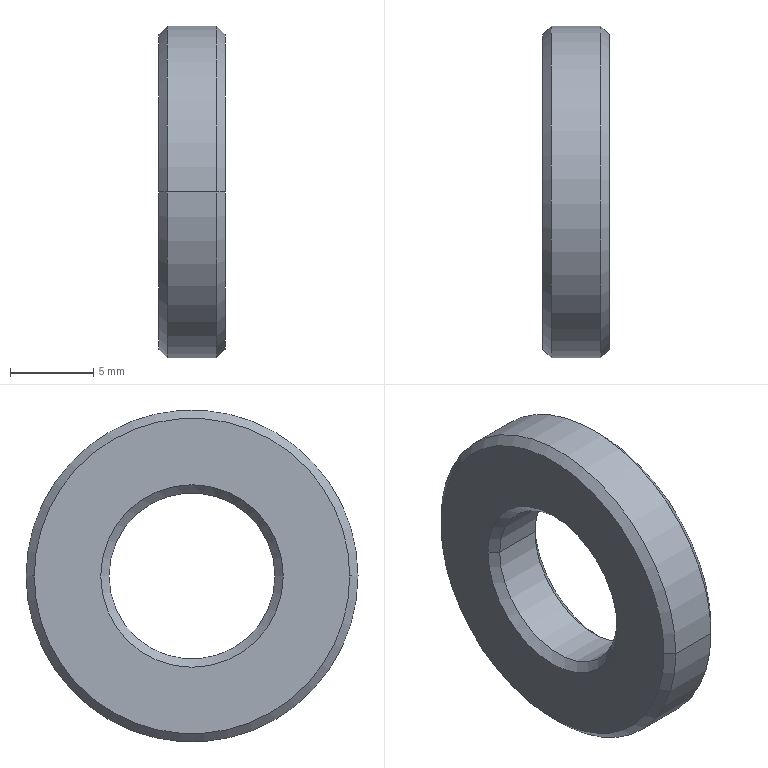Part | STEP file | WSSS20-10-4 | 1 solid | 14 faces | box 4 x 20 x 20 mm | volume 918.916 mm3 | cone 8 | cylinder 4 | plane 2 | commonest cylinder face diameters 10 x2 20 x2
STEP:
#1=CARTESIAN_POINT('',(0.,0.,0.));
#2=DIRECTION('',(0.,0.,1.));
#3=DIRECTION('',(1.,0.,0.));
#4=AXIS2_PLACEMENT_3D('',#1,#2,#3);
#5=CARTESIAN_POINT('',(3.5,-5.,0.));
#6=VERTEX_POINT('',#5);
#7=CARTESIAN_POINT('',(0.5,-5.,0.));
#8=VERTEX_POINT('',#7);
#9=CARTESIAN_POINT('',(-3.,-5.,0.));
#10=DIRECTION('',(-1.,0.,0.));
#11=VECTOR('',#10,1.);
#12=LINE('',#9,#11);
#13=CARTESIAN_POINT('',(-3.,0.,0.));
#14=DIRECTION('',(-1.,0.,0.));
#15=DIRECTION('',(0.,-1.,0.));
#16=AXIS2_PLACEMENT_3D('',#13,#14,#15);
#17=CYLINDRICAL_SURFACE('',#16,5.);
#18=CARTESIAN_POINT('',(6.283,0.));
#19=DIRECTION('',(0.,1.));
#20=VECTOR('',#19,1.);
#21=LINE('',#18,#20);
#22=(GEOMETRIC_REPRESENTATION_CONTEXT(2)PARAMETRIC_REPRESENTATION_CONTEXT()REPRESENTATION_CONTEXT('',''));
#23=DEFINITIONAL_REPRESENTATION('',(#21),#22);
#24=PCURVE('',#17,#23);
#25=CARTESIAN_POINT('',(-3.,0.,0.));
#26=DIRECTION('',(-1.,0.,0.));
#27=DIRECTION('',(0.,-1.,0.));
#28=AXIS2_PLACEMENT_3D('',#25,#26,#27);
#29=CYLINDRICAL_SURFACE('',#28,5.);
#30=CARTESIAN_POINT('',(0.,0.));
#31=DIRECTION('',(0.,1.));
#32=VECTOR('',#31,1.);
#33=LINE('',#30,#32);
#34=(GEOMETRIC_REPRESENTATION_CONTEXT(2)PARAMETRIC_REPRESENTATION_CONTEXT()REPRESENTATION_CONTEXT('',''));
#35=DEFINITIONAL_REPRESENTATION('',(#33),#34);
#36=PCURVE('',#29,#35);
#37=SURFACE_CURVE('',#12,(#24,#36),.PCURVE_S1.);
#38=EDGE_CURVE('',#6,#8,#37,.T.);
#39=ORIENTED_EDGE('',*,*,#38,.T.);
#40=CARTESIAN_POINT('',(0.5,5.,0.));
#41=VERTEX_POINT('',#40);
#42=CARTESIAN_POINT('',(0.5,0.,0.));
#43=DIRECTION('',(-1.,0.,0.));
#44=DIRECTION('',(0.,-1.,0.));
#45=AXIS2_PLACEMENT_3D('',#42,#43,#44);
#46=CIRCLE('',#45,5.);
#47=CARTESIAN_POINT('',(0.,-3.5));
#48=DIRECTION('',(1.,0.));
#49=VECTOR('',#48,1.);
#50=LINE('',#47,#49);
#51=(GEOMETRIC_REPRESENTATION_CONTEXT(2)PARAMETRIC_REPRESENTATION_CONTEXT()REPRESENTATION_CONTEXT('',''));
#52=DEFINITIONAL_REPRESENTATION('',(#50),#51);
#53=PCURVE('',#17,#52);
#54=CARTESIAN_POINT('',(0.5,0.,0.));
#55=DIRECTION('',(-1.,0.,0.));
#56=DIRECTION('',(0.,-1.,0.));
#57=AXIS2_PLACEMENT_3D('',#54,#55,#56);
#58=CONICAL_SURFACE('',#57,5.,0.7854);
#59=CARTESIAN_POINT('',(0.,0.));
#60=DIRECTION('',(1.,0.));
#61=VECTOR('',#60,1.);
#62=LINE('',#59,#61);
#63=(GEOMETRIC_REPRESENTATION_CONTEXT(2)PARAMETRIC_REPRESENTATION_CONTEXT()REPRESENTATION_CONTEXT('',''));
#64=DEFINITIONAL_REPRESENTATION('',(#62),#63);
#65=PCURVE('',#58,#64);
#66=SURFACE_CURVE('',#46,(#53,#65),.PCURVE_S1.);
#67=EDGE_CURVE('',#41,#8,#66,.T.);
#68=ORIENTED_EDGE('',*,*,#67,.F.);
#69=CARTESIAN_POINT('',(3.5,5.,0.));
#70=VERTEX_POINT('',#69);
#71=CARTESIAN_POINT('',(-3.,5.,0.));
#72=DIRECTION('',(-1.,0.,0.));
#73=VECTOR('',#72,1.);
#74=LINE('',#71,#73);
#75=CARTESIAN_POINT('',(3.142,0.));
#76=DIRECTION('',(0.,1.));
#77=VECTOR('',#76,1.);
#78=LINE('',#75,#77);
#79=(GEOMETRIC_REPRESENTATION_CONTEXT(2)PARAMETRIC_REPRESENTATION_CONTEXT()REPRESENTATION_CONTEXT('',''));
#80=DEFINITIONAL_REPRESENTATION('',(#78),#79);
#81=PCURVE('',#17,#80);
#82=CARTESIAN_POINT('',(3.142,0.));
#83=DIRECTION('',(0.,1.));
#84=VECTOR('',#83,1.);
#85=LINE('',#82,#84);
#86=(GEOMETRIC_REPRESENTATION_CONTEXT(2)PARAMETRIC_REPRESENTATION_CONTEXT()REPRESENTATION_CONTEXT('',''));
#87=DEFINITIONAL_REPRESENTATION('',(#85),#86);
#88=PCURVE('',#29,#87);
#89=SURFACE_CURVE('',#74,(#81,#88),.PCURVE_S1.);
#90=EDGE_CURVE('',#70,#41,#89,.T.);
#91=ORIENTED_EDGE('',*,*,#90,.F.);
#92=CARTESIAN_POINT('',(3.5,0.,0.));
#93=DIRECTION('',(-1.,0.,0.));
#94=DIRECTION('',(0.,-1.,0.));
#95=AXIS2_PLACEMENT_3D('',#92,#93,#94);
#96=CIRCLE('',#95,5.);
#97=CARTESIAN_POINT('',(0.,-6.5));
#98=DIRECTION('',(1.,0.));
#99=VECTOR('',#98,1.);
#100=LINE('',#97,#99);
#101=(GEOMETRIC_REPRESENTATION_CONTEXT(2)PARAMETRIC_REPRESENTATION_CONTEXT()REPRESENTATION_CONTEXT('',''));
#102=DEFINITIONAL_REPRESENTATION('',(#100),#101);
#103=PCURVE('',#17,#102);
#104=CARTESIAN_POINT('',(4.,0.,0.));
#105=DIRECTION('',(1.,0.,0.));
#106=DIRECTION('',(0.,1.,0.));
#107=AXIS2_PLACEMENT_3D('',#104,#105,#106);
#108=CONICAL_SURFACE('',#107,5.5,0.7854);
#109=CARTESIAN_POINT('',(9.425,-0.5));
#110=DIRECTION('',(-1.,0.));
#111=VECTOR('',#110,1.);
#112=LINE('',#109,#111);
#113=(GEOMETRIC_REPRESENTATION_CONTEXT(2)PARAMETRIC_REPRESENTATION_CONTEXT()REPRESENTATION_CONTEXT('',''));
#114=DEFINITIONAL_REPRESENTATION('',(#112),#113);
#115=PCURVE('',#108,#114);
#116=SURFACE_CURVE('',#96,(#103,#115),.PCURVE_S1.);
#117=EDGE_CURVE('',#70,#6,#116,.T.);
#118=ORIENTED_EDGE('',*,*,#117,.T.);
#119=EDGE_LOOP('',(#39,#68,#91,#118));
#120=FACE_BOUND('',#119,.F.);
#121=ADVANCED_FACE('',(#120),#17,.F.);
#122=CARTESIAN_POINT('',(4.,5.5,0.));
#123=VERTEX_POINT('',#122);
#124=CARTESIAN_POINT('',(4.,5.5,0.));
#125=DIRECTION('',(0.7071,0.7071,0.));
#126=VECTOR('',#125,1.);
#127=LINE('',#124,#126);
#128=CARTESIAN_POINT('',(6.283,0.));
#129=DIRECTION('',(0.,1.));
#130=VECTOR('',#129,1.);
#131=LINE('',#128,#130);
#132=(GEOMETRIC_REPRESENTATION_CONTEXT(2)PARAMETRIC_REPRESENTATION_CONTEXT()REPRESENTATION_CONTEXT('',''));
#133=DEFINITIONAL_REPRESENTATION('',(#131),#132);
#134=PCURVE('',#108,#133);
#135=CARTESIAN_POINT('',(4.,0.,0.));
#136=DIRECTION('',(1.,0.,0.));
#137=DIRECTION('',(0.,1.,0.));
#138=AXIS2_PLACEMENT_3D('',#135,#136,#137);
#139=CONICAL_SURFACE('',#138,5.5,0.7854);
#140=CARTESIAN_POINT('',(0.,0.));
#141=DIRECTION('',(0.,1.));
#142=VECTOR('',#141,1.);
#143=LINE('',#140,#142);
#144=(GEOMETRIC_REPRESENTATION_CONTEXT(2)PARAMETRIC_REPRESENTATION_CONTEXT()REPRESENTATION_CONTEXT('',''));
#145=DEFINITIONAL_REPRESENTATION('',(#143),#144);
#146=PCURVE('',#139,#145);
#147=SURFACE_CURVE('',#127,(#134,#146),.PCURVE_S1.);
#148=EDGE_CURVE('',#70,#123,#147,.T.);
#149=ORIENTED_EDGE('',*,*,#148,.T.);
#150=CARTESIAN_POINT('',(4.,-5.5,0.));
#151=VERTEX_POINT('',#150);
#152=CARTESIAN_POINT('',(4.,0.,0.));
#153=DIRECTION('',(-1.,0.,0.));
#154=DIRECTION('',(0.,-1.,0.));
#155=AXIS2_PLACEMENT_3D('',#152,#153,#154);
#156=CIRCLE('',#155,5.5);
#157=CARTESIAN_POINT('',(9.425,0.));
#158=DIRECTION('',(-1.,0.));
#159=VECTOR('',#158,1.);
#160=LINE('',#157,#159);
#161=(GEOMETRIC_REPRESENTATION_CONTEXT(2)PARAMETRIC_REPRESENTATION_CONTEXT()REPRESENTATION_CONTEXT('',''));
#162=DEFINITIONAL_REPRESENTATION('',(#160),#161);
#163=PCURVE('',#108,#162);
#164=CARTESIAN_POINT('',(4.,-9.5,0.));
#165=DIRECTION('',(1.,0.,0.));
#166=DIRECTION('',(0.,1.,0.));
#167=AXIS2_PLACEMENT_3D('',#164,#165,#166);
#168=PLANE('',#167);
#169=CARTESIAN_POINT('',(4.,0.));
#170=CARTESIAN_POINT('',(4.,9.526));
#171=CARTESIAN_POINT('',(12.25,4.763));
#172=CARTESIAN_POINT('',(20.5,0.));
#173=CARTESIAN_POINT('',(12.25,-4.763));
#174=CARTESIAN_POINT('',(4.,-9.526));
#175=CARTESIAN_POINT('',(4.,0.));
#176=(BOUNDED_CURVE()B_SPLINE_CURVE(2,(#169,#170,#171,#172,#173,#174,#175),.UNSPECIFIED.,.T.,.F.)B_SPLINE_CURVE_WITH_KNOTS((1,2,2,2,2,1),(-2.094,0.,2.094,4.189,6.283,8.378),.UNSPECIFIED.)CURVE()GEOMETRIC_REPRESENTATION_ITEM()RATIONAL_B_SPLINE_CURVE((1.,0.5,1.,0.5,1.,0.5,1.))REPRESENTATION_ITEM(''));
#177=(GEOMETRIC_REPRESENTATION_CONTEXT(2)PARAMETRIC_REPRESENTATION_CONTEXT()REPRESENTATION_CONTEXT('',''));
#178=DEFINITIONAL_REPRESENTATION('',(#176),#177);
#179=PCURVE('',#168,#178);
#180=SURFACE_CURVE('',#156,(#163,#179),.PCURVE_S1.);
#181=EDGE_CURVE('',#123,#151,#180,.T.);
#182=ORIENTED_EDGE('',*,*,#181,.T.);
#183=CARTESIAN_POINT('',(4.,-5.5,0.));
#184=DIRECTION('',(0.7071,-0.7071,0.));
#185=VECTOR('',#184,1.);
#186=LINE('',#183,#185);
#187=CARTESIAN_POINT('',(3.142,0.));
#188=DIRECTION('',(0.,1.));
#189=VECTOR('',#188,1.);
#190=LINE('',#187,#189);
#191=(GEOMETRIC_REPRESENTATION_CONTEXT(2)PARAMETRIC_REPRESENTATION_CONTEXT()REPRESENTATION_CONTEXT('',''));
#192=DEFINITIONAL_REPRESENTATION('',(#190),#191);
#193=PCURVE('',#108,#192);
#194=CARTESIAN_POINT('',(3.142,0.));
#195=DIRECTION('',(0.,1.));
#196=VECTOR('',#195,1.);
#197=LINE('',#194,#196);
#198=(GEOMETRIC_REPRESENTATION_CONTEXT(2)PARAMETRIC_REPRESENTATION_CONTEXT()REPRESENTATION_CONTEXT('',''));
#199=DEFINITIONAL_REPRESENTATION('',(#197),#198);
#200=PCURVE('',#139,#199);
#201=SURFACE_CURVE('',#186,(#193,#200),.PCURVE_S1.);
#202=EDGE_CURVE('',#6,#151,#201,.T.);
#203=ORIENTED_EDGE('',*,*,#202,.F.);
#204=ORIENTED_EDGE('',*,*,#117,.F.);
#205=EDGE_LOOP('',(#149,#182,#203,#204));
#206=FACE_BOUND('',#205,.F.);
#207=ADVANCED_FACE('',(#206),#108,.F.);
#208=CARTESIAN_POINT('',(4.,-9.5,0.));
#209=VERTEX_POINT('',#208);
#210=CARTESIAN_POINT('',(4.,9.5,0.));
#211=VERTEX_POINT('',#210);
#212=CARTESIAN_POINT('',(4.,0.,0.));
#213=DIRECTION('',(-1.,0.,0.));
#214=DIRECTION('',(0.,-1.,0.));
#215=AXIS2_PLACEMENT_3D('',#212,#213,#214);
#216=CIRCLE('',#215,9.5);
#217=CARTESIAN_POINT('',(3.5,0.,0.));
#218=DIRECTION('',(-1.,0.,0.));
#219=DIRECTION('',(0.,-1.,0.));
#220=AXIS2_PLACEMENT_3D('',#217,#218,#219);
#221=CONICAL_SURFACE('',#220,10.,0.7854);
#222=CARTESIAN_POINT('',(0.,-0.5));
#223=DIRECTION('',(1.,0.));
#224=VECTOR('',#223,1.);
#225=LINE('',#222,#224);
#226=(GEOMETRIC_REPRESENTATION_CONTEXT(2)PARAMETRIC_REPRESENTATION_CONTEXT()REPRESENTATION_CONTEXT('',''));
#227=DEFINITIONAL_REPRESENTATION('',(#225),#226);
#228=PCURVE('',#221,#227);
#229=CARTESIAN_POINT('',(0.,0.));
#230=CARTESIAN_POINT('',(0.,16.454));
#231=CARTESIAN_POINT('',(14.25,8.227));
#232=CARTESIAN_POINT('',(28.5,0.));
#233=CARTESIAN_POINT('',(14.25,-8.227));
#234=CARTESIAN_POINT('',(0.,-16.454));
#235=CARTESIAN_POINT('',(0.,0.));
#236=(BOUNDED_CURVE()B_SPLINE_CURVE(2,(#229,#230,#231,#232,#233,#234,#235),.UNSPECIFIED.,.T.,.F.)B_SPLINE_CURVE_WITH_KNOTS((1,2,2,2,2,1),(-2.094,0.,2.094,4.189,6.283,8.378),.UNSPECIFIED.)CURVE()GEOMETRIC_REPRESENTATION_ITEM()RATIONAL_B_SPLINE_CURVE((1.,0.5,1.,0.5,1.,0.5,1.))REPRESENTATION_ITEM(''));
#237=(GEOMETRIC_REPRESENTATION_CONTEXT(2)PARAMETRIC_REPRESENTATION_CONTEXT()REPRESENTATION_CONTEXT('',''));
#238=DEFINITIONAL_REPRESENTATION('',(#236),#237);
#239=PCURVE('',#168,#238);
#240=SURFACE_CURVE('',#216,(#228,#239),.PCURVE_S1.);
#241=EDGE_CURVE('',#209,#211,#240,.T.);
#242=ORIENTED_EDGE('',*,*,#241,.T.);
#243=CARTESIAN_POINT('',(3.5,10.,0.));
#244=VERTEX_POINT('',#243);
#245=CARTESIAN_POINT('',(3.5,10.,0.));
#246=DIRECTION('',(-0.7071,0.7071,0.));
#247=VECTOR('',#246,1.);
#248=LINE('',#245,#247);
#249=CARTESIAN_POINT('',(3.142,0.));
#250=DIRECTION('',(0.,1.));
#251=VECTOR('',#250,1.);
#252=LINE('',#249,#251);
#253=(GEOMETRIC_REPRESENTATION_CONTEXT(2)PARAMETRIC_REPRESENTATION_CONTEXT()REPRESENTATION_CONTEXT('',''));
#254=DEFINITIONAL_REPRESENTATION('',(#252),#253);
#255=PCURVE('',#221,#254);
#256=CARTESIAN_POINT('',(3.5,0.,0.));
#257=DIRECTION('',(-1.,0.,0.));
#258=DIRECTION('',(0.,-1.,0.));
#259=AXIS2_PLACEMENT_3D('',#256,#257,#258);
#260=CONICAL_SURFACE('',#259,10.,0.7854);
#261=CARTESIAN_POINT('',(3.142,0.));
#262=DIRECTION('',(0.,1.));
#263=VECTOR('',#262,1.);
#264=LINE('',#261,#263);
#265=(GEOMETRIC_REPRESENTATION_CONTEXT(2)PARAMETRIC_REPRESENTATION_CONTEXT()REPRESENTATION_CONTEXT('',''));
#266=DEFINITIONAL_REPRESENTATION('',(#264),#265);
#267=PCURVE('',#260,#266);
#268=SURFACE_CURVE('',#248,(#255,#267),.PCURVE_S1.);
#269=EDGE_CURVE('',#211,#244,#268,.T.);
#270=ORIENTED_EDGE('',*,*,#269,.T.);
#271=CARTESIAN_POINT('',(3.5,-10.,0.));
#272=VERTEX_POINT('',#271);
#273=CARTESIAN_POINT('',(3.5,0.,0.));
#274=DIRECTION('',(-1.,0.,0.));
#275=DIRECTION('',(0.,-1.,0.));
#276=AXIS2_PLACEMENT_3D('',#273,#274,#275);
#277=CIRCLE('',#276,10.);
#278=CARTESIAN_POINT('',(0.,0.));
#279=DIRECTION('',(1.,0.));
#280=VECTOR('',#279,1.);
#281=LINE('',#278,#280);
#282=(GEOMETRIC_REPRESENTATION_CONTEXT(2)PARAMETRIC_REPRESENTATION_CONTEXT()REPRESENTATION_CONTEXT('',''));
#283=DEFINITIONAL_REPRESENTATION('',(#281),#282);
#284=PCURVE('',#221,#283);
#285=CARTESIAN_POINT('',(-3.,0.,0.));
#286=DIRECTION('',(-1.,0.,0.));
#287=DIRECTION('',(0.,-1.,0.));
#288=AXIS2_PLACEMENT_3D('',#285,#286,#287);
#289=CYLINDRICAL_SURFACE('',#288,10.);
#290=CARTESIAN_POINT('',(0.,-6.5));
#291=DIRECTION('',(1.,0.));
#292=VECTOR('',#291,1.);
#293=LINE('',#290,#292);
#294=(GEOMETRIC_REPRESENTATION_CONTEXT(2)PARAMETRIC_REPRESENTATION_CONTEXT()REPRESENTATION_CONTEXT('',''));
#295=DEFINITIONAL_REPRESENTATION('',(#293),#294);
#296=PCURVE('',#289,#295);
#297=SURFACE_CURVE('',#277,(#284,#296),.PCURVE_S1.);
#298=EDGE_CURVE('',#272,#244,#297,.T.);
#299=ORIENTED_EDGE('',*,*,#298,.F.);
#300=CARTESIAN_POINT('',(3.5,-10.,0.));
#301=DIRECTION('',(-0.7071,-0.7071,0.));
#302=VECTOR('',#301,1.);
#303=LINE('',#300,#302);
#304=CARTESIAN_POINT('',(0.,0.));
#305=DIRECTION('',(0.,1.));
#306=VECTOR('',#305,1.);
#307=LINE('',#304,#306);
#308=(GEOMETRIC_REPRESENTATION_CONTEXT(2)PARAMETRIC_REPRESENTATION_CONTEXT()REPRESENTATION_CONTEXT('',''));
#309=DEFINITIONAL_REPRESENTATION('',(#307),#308);
#310=PCURVE('',#221,#309);
#311=CARTESIAN_POINT('',(6.283,0.));
#312=DIRECTION('',(0.,1.));
#313=VECTOR('',#312,1.);
#314=LINE('',#311,#313);
#315=(GEOMETRIC_REPRESENTATION_CONTEXT(2)PARAMETRIC_REPRESENTATION_CONTEXT()REPRESENTATION_CONTEXT('',''));
#316=DEFINITIONAL_REPRESENTATION('',(#314),#315);
#317=PCURVE('',#260,#316);
#318=SURFACE_CURVE('',#303,(#310,#317),.PCURVE_S1.);
#319=EDGE_CURVE('',#209,#272,#318,.T.);
#320=ORIENTED_EDGE('',*,*,#319,.F.);
#321=EDGE_LOOP('',(#242,#270,#299,#320));
#322=FACE_BOUND('',#321,.T.);
#323=ADVANCED_FACE('',(#322),#221,.T.);
#324=ORIENTED_EDGE('',*,*,#298,.T.);
#325=CARTESIAN_POINT('',(0.5,10.,0.));
#326=VERTEX_POINT('',#325);
#327=CARTESIAN_POINT('',(-3.,10.,0.));
#328=DIRECTION('',(-1.,0.,0.));
#329=VECTOR('',#328,1.);
#330=LINE('',#327,#329);
#331=CARTESIAN_POINT('',(3.142,0.));
#332=DIRECTION('',(0.,1.));
#333=VECTOR('',#332,1.);
#334=LINE('',#331,#333);
#335=(GEOMETRIC_REPRESENTATION_CONTEXT(2)PARAMETRIC_REPRESENTATION_CONTEXT()REPRESENTATION_CONTEXT('',''));
#336=DEFINITIONAL_REPRESENTATION('',(#334),#335);
#337=PCURVE('',#289,#336);
#338=CARTESIAN_POINT('',(-3.,0.,0.));
#339=DIRECTION('',(-1.,0.,0.));
#340=DIRECTION('',(0.,-1.,0.));
#341=AXIS2_PLACEMENT_3D('',#338,#339,#340);
#342=CYLINDRICAL_SURFACE('',#341,10.);
#343=CARTESIAN_POINT('',(3.142,0.));
#344=DIRECTION('',(0.,1.));
#345=VECTOR('',#344,1.);
#346=LINE('',#343,#345);
#347=(GEOMETRIC_REPRESENTATION_CONTEXT(2)PARAMETRIC_REPRESENTATION_CONTEXT()REPRESENTATION_CONTEXT('',''));
#348=DEFINITIONAL_REPRESENTATION('',(#346),#347);
#349=PCURVE('',#342,#348);
#350=SURFACE_CURVE('',#330,(#337,#349),.PCURVE_S1.);
#351=EDGE_CURVE('',#244,#326,#350,.T.);
#352=ORIENTED_EDGE('',*,*,#351,.T.);
#353=CARTESIAN_POINT('',(0.5,-10.,0.));
#354=VERTEX_POINT('',#353);
#355=CARTESIAN_POINT('',(0.5,0.,0.));
#356=DIRECTION('',(-1.,0.,0.));
#357=DIRECTION('',(0.,-1.,0.));
#358=AXIS2_PLACEMENT_3D('',#355,#356,#357);
#359=CIRCLE('',#358,10.);
#360=CARTESIAN_POINT('',(0.,-3.5));
#361=DIRECTION('',(1.,0.));
#362=VECTOR('',#361,1.);
#363=LINE('',#360,#362);
#364=(GEOMETRIC_REPRESENTATION_CONTEXT(2)PARAMETRIC_REPRESENTATION_CONTEXT()REPRESENTATION_CONTEXT('',''));
#365=DEFINITIONAL_REPRESENTATION('',(#363),#364);
#366=PCURVE('',#289,#365);
#367=CARTESIAN_POINT('',(0.,0.,0.));
#368=DIRECTION('',(1.,0.,0.));
#369=DIRECTION('',(0.,1.,0.));
#370=AXIS2_PLACEMENT_3D('',#367,#368,#369);
#371=CONICAL_SURFACE('',#370,9.5,0.7854);
#372=CARTESIAN_POINT('',(3.142,0.5));
#373=DIRECTION('',(-1.,0.));
#374=VECTOR('',#373,1.);
#375=LINE('',#372,#374);
#376=(GEOMETRIC_REPRESENTATION_CONTEXT(2)PARAMETRIC_REPRESENTATION_CONTEXT()REPRESENTATION_CONTEXT('',''));
#377=DEFINITIONAL_REPRESENTATION('',(#375),#376);
#378=PCURVE('',#371,#377);
#379=SURFACE_CURVE('',#359,(#366,#378),.PCURVE_S1.);
#380=EDGE_CURVE('',#354,#326,#379,.T.);
#381=ORIENTED_EDGE('',*,*,#380,.F.);
#382=CARTESIAN_POINT('',(-3.,-10.,0.));
#383=DIRECTION('',(-1.,0.,0.));
#384=VECTOR('',#383,1.);
#385=LINE('',#382,#384);
#386=CARTESIAN_POINT('',(0.,0.));
#387=DIRECTION('',(0.,1.));
#388=VECTOR('',#387,1.);
#389=LINE('',#386,#388);
#390=(GEOMETRIC_REPRESENTATION_CONTEXT(2)PARAMETRIC_REPRESENTATION_CONTEXT()REPRESENTATION_CONTEXT('',''));
#391=DEFINITIONAL_REPRESENTATION('',(#389),#390);
#392=PCURVE('',#289,#391);
#393=CARTESIAN_POINT('',(6.283,0.));
#394=DIRECTION('',(0.,1.));
#395=VECTOR('',#394,1.);
#396=LINE('',#393,#395);
#397=(GEOMETRIC_REPRESENTATION_CONTEXT(2)PARAMETRIC_REPRESENTATION_CONTEXT()REPRESENTATION_CONTEXT('',''));
#398=DEFINITIONAL_REPRESENTATION('',(#396),#397);
#399=PCURVE('',#342,#398);
#400=SURFACE_CURVE('',#385,(#392,#399),.PCURVE_S1.);
#401=EDGE_CURVE('',#272,#354,#400,.T.);
#402=ORIENTED_EDGE('',*,*,#401,.F.);
#403=EDGE_LOOP('',(#324,#352,#381,#402));
#404=FACE_BOUND('',#403,.T.);
#405=ADVANCED_FACE('',(#404),#289,.T.);
#406=CARTESIAN_POINT('',(0.,-9.5,0.));
#407=VERTEX_POINT('',#406);
#408=CARTESIAN_POINT('',(0.,9.5,0.));
#409=VERTEX_POINT('',#408);
#410=CARTESIAN_POINT('',(0.,0.,0.));
#411=DIRECTION('',(-1.,0.,0.));
#412=DIRECTION('',(0.,-1.,0.));
#413=AXIS2_PLACEMENT_3D('',#410,#411,#412);
#414=CIRCLE('',#413,9.5);
#415=CARTESIAN_POINT('',(3.142,0.));
#416=DIRECTION('',(-1.,0.));
#417=VECTOR('',#416,1.);
#418=LINE('',#415,#417);
#419=(GEOMETRIC_REPRESENTATION_CONTEXT(2)PARAMETRIC_REPRESENTATION_CONTEXT()REPRESENTATION_CONTEXT('',''));
#420=DEFINITIONAL_REPRESENTATION('',(#418),#419);
#421=PCURVE('',#371,#420);
#422=CARTESIAN_POINT('',(0.,-5.5,0.));
#423=DIRECTION('',(-1.,0.,0.));
#424=DIRECTION('',(0.,-1.,0.));
#425=AXIS2_PLACEMENT_3D('',#422,#423,#424);
#426=PLANE('',#425);
#427=CARTESIAN_POINT('',(-5.5,0.));
#428=DIRECTION('',(1.,0.));
#429=AXIS2_PLACEMENT_2D('',#427,#428);
#430=CIRCLE('',#429,9.5);
#431=(GEOMETRIC_REPRESENTATION_CONTEXT(2)PARAMETRIC_REPRESENTATION_CONTEXT()REPRESENTATION_CONTEXT('',''));
#432=DEFINITIONAL_REPRESENTATION('',(#430),#431);
#433=PCURVE('',#426,#432);
#434=SURFACE_CURVE('',#414,(#421,#433),.PCURVE_S1.);
#435=EDGE_CURVE('',#407,#409,#434,.T.);
#436=ORIENTED_EDGE('',*,*,#435,.F.);
#437=CARTESIAN_POINT('',(0.,-9.5,0.));
#438=DIRECTION('',(0.7071,-0.7071,0.));
#439=VECTOR('',#438,1.);
#440=LINE('',#437,#439);
#441=CARTESIAN_POINT('',(3.142,0.));
#442=DIRECTION('',(0.,1.));
#443=VECTOR('',#442,1.);
#444=LINE('',#441,#443);
#445=(GEOMETRIC_REPRESENTATION_CONTEXT(2)PARAMETRIC_REPRESENTATION_CONTEXT()REPRESENTATION_CONTEXT('',''));
#446=DEFINITIONAL_REPRESENTATION('',(#444),#445);
#447=PCURVE('',#371,#446);
#448=CARTESIAN_POINT('',(0.,0.,0.));
#449=DIRECTION('',(1.,0.,0.));
#450=DIRECTION('',(0.,1.,0.));
#451=AXIS2_PLACEMENT_3D('',#448,#449,#450);
#452=CONICAL_SURFACE('',#451,9.5,0.7854);
#453=CARTESIAN_POINT('',(3.142,0.));
#454=DIRECTION('',(0.,1.));
#455=VECTOR('',#454,1.);
#456=LINE('',#453,#455);
#457=(GEOMETRIC_REPRESENTATION_CONTEXT(2)PARAMETRIC_REPRESENTATION_CONTEXT()REPRESENTATION_CONTEXT('',''));
#458=DEFINITIONAL_REPRESENTATION('',(#456),#457);
#459=PCURVE('',#452,#458);
#460=SURFACE_CURVE('',#440,(#447,#459),.PCURVE_S1.);
#461=EDGE_CURVE('',#407,#354,#460,.T.);
#462=ORIENTED_EDGE('',*,*,#461,.T.);
#463=ORIENTED_EDGE('',*,*,#380,.T.);
#464=CARTESIAN_POINT('',(0.,9.5,0.));
#465=DIRECTION('',(0.7071,0.7071,0.));
#466=VECTOR('',#465,1.);
#467=LINE('',#464,#466);
#468=CARTESIAN_POINT('',(0.,0.));
#469=DIRECTION('',(0.,1.));
#470=VECTOR('',#469,1.);
#471=LINE('',#468,#470);
#472=(GEOMETRIC_REPRESENTATION_CONTEXT(2)PARAMETRIC_REPRESENTATION_CONTEXT()REPRESENTATION_CONTEXT('',''));
#473=DEFINITIONAL_REPRESENTATION('',(#471),#472);
#474=PCURVE('',#371,#473);
#475=CARTESIAN_POINT('',(6.283,0.));
#476=DIRECTION('',(0.,1.));
#477=VECTOR('',#476,1.);
#478=LINE('',#475,#477);
#479=(GEOMETRIC_REPRESENTATION_CONTEXT(2)PARAMETRIC_REPRESENTATION_CONTEXT()REPRESENTATION_CONTEXT('',''));
#480=DEFINITIONAL_REPRESENTATION('',(#478),#479);
#481=PCURVE('',#452,#480);
#482=SURFACE_CURVE('',#467,(#474,#481),.PCURVE_S1.);
#483=EDGE_CURVE('',#409,#326,#482,.T.);
#484=ORIENTED_EDGE('',*,*,#483,.F.);
#485=EDGE_LOOP('',(#436,#462,#463,#484));
#486=FACE_BOUND('',#485,.T.);
#487=ADVANCED_FACE('',(#486),#371,.T.);
#488=CARTESIAN_POINT('',(0.,-5.5,0.));
#489=VERTEX_POINT('',#488);
#490=CARTESIAN_POINT('',(0.5,-5.,0.));
#491=DIRECTION('',(-0.7071,-0.7071,0.));
#492=VECTOR('',#491,1.);
#493=LINE('',#490,#492);
#494=CARTESIAN_POINT('',(6.283,0.));
#495=DIRECTION('',(0.,1.));
#496=VECTOR('',#495,1.);
#497=LINE('',#494,#496);
#498=(GEOMETRIC_REPRESENTATION_CONTEXT(2)PARAMETRIC_REPRESENTATION_CONTEXT()REPRESENTATION_CONTEXT('',''));
#499=DEFINITIONAL_REPRESENTATION('',(#497),#498);
#500=PCURVE('',#58,#499);
#501=CARTESIAN_POINT('',(0.5,0.,0.));
#502=DIRECTION('',(-1.,0.,0.));
#503=DIRECTION('',(0.,-1.,0.));
#504=AXIS2_PLACEMENT_3D('',#501,#502,#503);
#505=CONICAL_SURFACE('',#504,5.,0.7854);
#506=CARTESIAN_POINT('',(0.,0.));
#507=DIRECTION('',(0.,1.));
#508=VECTOR('',#507,1.);
#509=LINE('',#506,#508);
#510=(GEOMETRIC_REPRESENTATION_CONTEXT(2)PARAMETRIC_REPRESENTATION_CONTEXT()REPRESENTATION_CONTEXT('',''));
#511=DEFINITIONAL_REPRESENTATION('',(#509),#510);
#512=PCURVE('',#505,#511);
#513=SURFACE_CURVE('',#493,(#500,#512),.PCURVE_S1.);
#514=EDGE_CURVE('',#8,#489,#513,.T.);
#515=ORIENTED_EDGE('',*,*,#514,.T.);
#516=CARTESIAN_POINT('',(0.,5.5,0.));
#517=VERTEX_POINT('',#516);
#518=CARTESIAN_POINT('',(0.,0.,0.));
#519=DIRECTION('',(-1.,0.,0.));
#520=DIRECTION('',(0.,-1.,0.));
#521=AXIS2_PLACEMENT_3D('',#518,#519,#520);
#522=CIRCLE('',#521,5.5);
#523=CARTESIAN_POINT('',(0.,0.5));
#524=DIRECTION('',(1.,0.));
#525=VECTOR('',#524,1.);
#526=LINE('',#523,#525);
#527=(GEOMETRIC_REPRESENTATION_CONTEXT(2)PARAMETRIC_REPRESENTATION_CONTEXT()REPRESENTATION_CONTEXT('',''));
#528=DEFINITIONAL_REPRESENTATION('',(#526),#527);
#529=PCURVE('',#58,#528);
#530=CARTESIAN_POINT('',(-5.5,0.));
#531=DIRECTION('',(1.,0.));
#532=AXIS2_PLACEMENT_2D('',#530,#531);
#533=CIRCLE('',#532,5.5);
#534=(GEOMETRIC_REPRESENTATION_CONTEXT(2)PARAMETRIC_REPRESENTATION_CONTEXT()REPRESENTATION_CONTEXT('',''));
#535=DEFINITIONAL_REPRESENTATION('',(#533),#534);
#536=PCURVE('',#426,#535);
#537=SURFACE_CURVE('',#522,(#529,#536),.PCURVE_S1.);
#538=EDGE_CURVE('',#517,#489,#537,.T.);
#539=ORIENTED_EDGE('',*,*,#538,.F.);
#540=CARTESIAN_POINT('',(0.5,5.,0.));
#541=DIRECTION('',(-0.7071,0.7071,0.));
#542=VECTOR('',#541,1.);
#543=LINE('',#540,#542);
#544=CARTESIAN_POINT('',(3.142,0.));
#545=DIRECTION('',(0.,1.));
#546=VECTOR('',#545,1.);
#547=LINE('',#544,#546);
#548=(GEOMETRIC_REPRESENTATION_CONTEXT(2)PARAMETRIC_REPRESENTATION_CONTEXT()REPRESENTATION_CONTEXT('',''));
#549=DEFINITIONAL_REPRESENTATION('',(#547),#548);
#550=PCURVE('',#58,#549);
#551=CARTESIAN_POINT('',(3.142,0.));
#552=DIRECTION('',(0.,1.));
#553=VECTOR('',#552,1.);
#554=LINE('',#551,#553);
#555=(GEOMETRIC_REPRESENTATION_CONTEXT(2)PARAMETRIC_REPRESENTATION_CONTEXT()REPRESENTATION_CONTEXT('',''));
#556=DEFINITIONAL_REPRESENTATION('',(#554),#555);
#557=PCURVE('',#505,#556);
#558=SURFACE_CURVE('',#543,(#550,#557),.PCURVE_S1.);
#559=EDGE_CURVE('',#41,#517,#558,.T.);
#560=ORIENTED_EDGE('',*,*,#559,.F.);
#561=ORIENTED_EDGE('',*,*,#67,.T.);
#562=EDGE_LOOP('',(#515,#539,#560,#561));
#563=FACE_BOUND('',#562,.F.);
#564=ADVANCED_FACE('',(#563),#58,.F.);
#565=CARTESIAN_POINT('',(0.,0.,0.));
#566=DIRECTION('',(-1.,0.,0.));
#567=DIRECTION('',(0.,-1.,0.));
#568=AXIS2_PLACEMENT_3D('',#565,#566,#567);
#569=CIRCLE('',#568,5.5);
#570=CARTESIAN_POINT('',(0.,0.5));
#571=DIRECTION('',(1.,0.));
#572=VECTOR('',#571,1.);
#573=LINE('',#570,#572);
#574=(GEOMETRIC_REPRESENTATION_CONTEXT(2)PARAMETRIC_REPRESENTATION_CONTEXT()REPRESENTATION_CONTEXT('',''));
#575=DEFINITIONAL_REPRESENTATION('',(#573),#574);
#576=PCURVE('',#505,#575);
#577=CARTESIAN_POINT('',(-5.5,0.));
#578=DIRECTION('',(1.,0.));
#579=AXIS2_PLACEMENT_2D('',#577,#578);
#580=CIRCLE('',#579,5.5);
#581=(GEOMETRIC_REPRESENTATION_CONTEXT(2)PARAMETRIC_REPRESENTATION_CONTEXT()REPRESENTATION_CONTEXT('',''));
#582=DEFINITIONAL_REPRESENTATION('',(#580),#581);
#583=PCURVE('',#426,#582);
#584=SURFACE_CURVE('',#569,(#576,#583),.PCURVE_S1.);
#585=EDGE_CURVE('',#489,#517,#584,.T.);
#586=ORIENTED_EDGE('',*,*,#585,.F.);
#587=ORIENTED_EDGE('',*,*,#514,.F.);
#588=CARTESIAN_POINT('',(0.5,0.,0.));
#589=DIRECTION('',(-1.,0.,0.));
#590=DIRECTION('',(0.,-1.,0.));
#591=AXIS2_PLACEMENT_3D('',#588,#589,#590);
#592=CIRCLE('',#591,5.);
#593=CARTESIAN_POINT('',(0.,0.));
#594=DIRECTION('',(1.,0.));
#595=VECTOR('',#594,1.);
#596=LINE('',#593,#595);
#597=(GEOMETRIC_REPRESENTATION_CONTEXT(2)PARAMETRIC_REPRESENTATION_CONTEXT()REPRESENTATION_CONTEXT('',''));
#598=DEFINITIONAL_REPRESENTATION('',(#596),#597);
#599=PCURVE('',#505,#598);
#600=CARTESIAN_POINT('',(0.,-3.5));
#601=DIRECTION('',(1.,0.));
#602=VECTOR('',#601,1.);
#603=LINE('',#600,#602);
#604=(GEOMETRIC_REPRESENTATION_CONTEXT(2)PARAMETRIC_REPRESENTATION_CONTEXT()REPRESENTATION_CONTEXT('',''));
#605=DEFINITIONAL_REPRESENTATION('',(#603),#604);
#606=PCURVE('',#29,#605);
#607=SURFACE_CURVE('',#592,(#599,#606),.PCURVE_S1.);
#608=EDGE_CURVE('',#8,#41,#607,.T.);
#609=ORIENTED_EDGE('',*,*,#608,.T.);
#610=ORIENTED_EDGE('',*,*,#559,.T.);
#611=EDGE_LOOP('',(#586,#587,#609,#610));
#612=FACE_BOUND('',#611,.F.);
#613=ADVANCED_FACE('',(#612),#505,.F.);
#614=CARTESIAN_POINT('',(0.,0.,0.));
#615=DIRECTION('',(-1.,0.,0.));
#616=DIRECTION('',(0.,-1.,0.));
#617=AXIS2_PLACEMENT_3D('',#614,#615,#616);
#618=CIRCLE('',#617,9.5);
#619=CARTESIAN_POINT('',(-5.5,0.));
#620=DIRECTION('',(1.,0.));
#621=AXIS2_PLACEMENT_2D('',#619,#620);
#622=CIRCLE('',#621,9.5);
#623=(GEOMETRIC_REPRESENTATION_CONTEXT(2)PARAMETRIC_REPRESENTATION_CONTEXT()REPRESENTATION_CONTEXT('',''));
#624=DEFINITIONAL_REPRESENTATION('',(#622),#623);
#625=PCURVE('',#426,#624);
#626=CARTESIAN_POINT('',(9.425,0.));
#627=DIRECTION('',(-1.,0.));
#628=VECTOR('',#627,1.);
#629=LINE('',#626,#628);
#630=(GEOMETRIC_REPRESENTATION_CONTEXT(2)PARAMETRIC_REPRESENTATION_CONTEXT()REPRESENTATION_CONTEXT('',''));
#631=DEFINITIONAL_REPRESENTATION('',(#629),#630);
#632=PCURVE('',#452,#631);
#633=SURFACE_CURVE('',#618,(#625,#632),.PCURVE_S1.);
#634=EDGE_CURVE('',#409,#407,#633,.T.);
#635=ORIENTED_EDGE('',*,*,#634,.T.);
#636=ORIENTED_EDGE('',*,*,#435,.T.);
#637=EDGE_LOOP('',(#635,#636));
#638=FACE_BOUND('',#637,.T.);
#639=ORIENTED_EDGE('',*,*,#585,.F.);
#640=ORIENTED_EDGE('',*,*,#538,.F.);
#641=EDGE_LOOP('',(#639,#640));
#642=FACE_BOUND('',#641,.T.);
#643=ADVANCED_FACE('',(#638,#642),#426,.T.);
#644=ORIENTED_EDGE('',*,*,#461,.F.);
#645=ORIENTED_EDGE('',*,*,#634,.F.);
#646=ORIENTED_EDGE('',*,*,#483,.T.);
#647=CARTESIAN_POINT('',(0.5,0.,0.));
#648=DIRECTION('',(-1.,0.,0.));
#649=DIRECTION('',(0.,-1.,0.));
#650=AXIS2_PLACEMENT_3D('',#647,#648,#649);
#651=CIRCLE('',#650,10.);
#652=CARTESIAN_POINT('',(9.425,0.5));
#653=DIRECTION('',(-1.,0.));
#654=VECTOR('',#653,1.);
#655=LINE('',#652,#654);
#656=(GEOMETRIC_REPRESENTATION_CONTEXT(2)PARAMETRIC_REPRESENTATION_CONTEXT()REPRESENTATION_CONTEXT('',''));
#657=DEFINITIONAL_REPRESENTATION('',(#655),#656);
#658=PCURVE('',#452,#657);
#659=CARTESIAN_POINT('',(0.,-3.5));
#660=DIRECTION('',(1.,0.));
#661=VECTOR('',#660,1.);
#662=LINE('',#659,#661);
#663=(GEOMETRIC_REPRESENTATION_CONTEXT(2)PARAMETRIC_REPRESENTATION_CONTEXT()REPRESENTATION_CONTEXT('',''));
#664=DEFINITIONAL_REPRESENTATION('',(#662),#663);
#665=PCURVE('',#342,#664);
#666=SURFACE_CURVE('',#651,(#658,#665),.PCURVE_S1.);
#667=EDGE_CURVE('',#326,#354,#666,.T.);
#668=ORIENTED_EDGE('',*,*,#667,.T.);
#669=EDGE_LOOP('',(#644,#645,#646,#668));
#670=FACE_BOUND('',#669,.T.);
#671=ADVANCED_FACE('',(#670),#452,.T.);
#672=ORIENTED_EDGE('',*,*,#351,.F.);
#673=CARTESIAN_POINT('',(3.5,0.,0.));
#674=DIRECTION('',(-1.,0.,0.));
#675=DIRECTION('',(0.,-1.,0.));
#676=AXIS2_PLACEMENT_3D('',#673,#674,#675);
#677=CIRCLE('',#676,10.);
#678=CARTESIAN_POINT('',(0.,-6.5));
#679=DIRECTION('',(1.,0.));
#680=VECTOR('',#679,1.);
#681=LINE('',#678,#680);
#682=(GEOMETRIC_REPRESENTATION_CONTEXT(2)PARAMETRIC_REPRESENTATION_CONTEXT()REPRESENTATION_CONTEXT('',''));
#683=DEFINITIONAL_REPRESENTATION('',(#681),#682);
#684=PCURVE('',#342,#683);
#685=CARTESIAN_POINT('',(0.,0.));
#686=DIRECTION('',(1.,0.));
#687=VECTOR('',#686,1.);
#688=LINE('',#685,#687);
#689=(GEOMETRIC_REPRESENTATION_CONTEXT(2)PARAMETRIC_REPRESENTATION_CONTEXT()REPRESENTATION_CONTEXT('',''));
#690=DEFINITIONAL_REPRESENTATION('',(#688),#689);
#691=PCURVE('',#260,#690);
#692=SURFACE_CURVE('',#677,(#684,#691),.PCURVE_S1.);
#693=EDGE_CURVE('',#244,#272,#692,.T.);
#694=ORIENTED_EDGE('',*,*,#693,.T.);
#695=ORIENTED_EDGE('',*,*,#401,.T.);
#696=ORIENTED_EDGE('',*,*,#667,.F.);
#697=EDGE_LOOP('',(#672,#694,#695,#696));
#698=FACE_BOUND('',#697,.T.);
#699=ADVANCED_FACE('',(#698),#342,.T.);
#700=ORIENTED_EDGE('',*,*,#269,.F.);
#701=CARTESIAN_POINT('',(4.,0.,0.));
#702=DIRECTION('',(-1.,0.,0.));
#703=DIRECTION('',(0.,-1.,0.));
#704=AXIS2_PLACEMENT_3D('',#701,#702,#703);
#705=CIRCLE('',#704,9.5);
#706=CARTESIAN_POINT('',(0.,-0.5));
#707=DIRECTION('',(1.,0.));
#708=VECTOR('',#707,1.);
#709=LINE('',#706,#708);
#710=(GEOMETRIC_REPRESENTATION_CONTEXT(2)PARAMETRIC_REPRESENTATION_CONTEXT()REPRESENTATION_CONTEXT('',''));
#711=DEFINITIONAL_REPRESENTATION('',(#709),#710);
#712=PCURVE('',#260,#711);
#713=CARTESIAN_POINT('',(0.,0.));
#714=CARTESIAN_POINT('',(0.,16.454));
#715=CARTESIAN_POINT('',(14.25,8.227));
#716=CARTESIAN_POINT('',(28.5,0.));
#717=CARTESIAN_POINT('',(14.25,-8.227));
#718=CARTESIAN_POINT('',(0.,-16.454));
#719=CARTESIAN_POINT('',(0.,0.));
#720=(BOUNDED_CURVE()B_SPLINE_CURVE(2,(#713,#714,#715,#716,#717,#718,#719),.UNSPECIFIED.,.T.,.F.)B_SPLINE_CURVE_WITH_KNOTS((1,2,2,2,2,1),(-2.094,0.,2.094,4.189,6.283,8.378),.UNSPECIFIED.)CURVE()GEOMETRIC_REPRESENTATION_ITEM()RATIONAL_B_SPLINE_CURVE((1.,0.5,1.,0.5,1.,0.5,1.))REPRESENTATION_ITEM(''));
#721=(GEOMETRIC_REPRESENTATION_CONTEXT(2)PARAMETRIC_REPRESENTATION_CONTEXT()REPRESENTATION_CONTEXT('',''));
#722=DEFINITIONAL_REPRESENTATION('',(#720),#721);
#723=PCURVE('',#168,#722);
#724=SURFACE_CURVE('',#705,(#712,#723),.PCURVE_S1.);
#725=EDGE_CURVE('',#211,#209,#724,.T.);
#726=ORIENTED_EDGE('',*,*,#725,.T.);
#727=ORIENTED_EDGE('',*,*,#319,.T.);
#728=ORIENTED_EDGE('',*,*,#693,.F.);
#729=EDGE_LOOP('',(#700,#726,#727,#728));
#730=FACE_BOUND('',#729,.T.);
#731=ADVANCED_FACE('',(#730),#260,.T.);
#732=ORIENTED_EDGE('',*,*,#181,.T.);
#733=CARTESIAN_POINT('',(4.,0.,0.));
#734=DIRECTION('',(-1.,0.,0.));
#735=DIRECTION('',(0.,-1.,0.));
#736=AXIS2_PLACEMENT_3D('',#733,#734,#735);
#737=CIRCLE('',#736,5.5);
#738=CARTESIAN_POINT('',(4.,0.));
#739=CARTESIAN_POINT('',(4.,9.526));
#740=CARTESIAN_POINT('',(12.25,4.763));
#741=CARTESIAN_POINT('',(20.5,0.));
#742=CARTESIAN_POINT('',(12.25,-4.763));
#743=CARTESIAN_POINT('',(4.,-9.526));
#744=CARTESIAN_POINT('',(4.,0.));
#745=(BOUNDED_CURVE()B_SPLINE_CURVE(2,(#738,#739,#740,#741,#742,#743,#744),.UNSPECIFIED.,.T.,.F.)B_SPLINE_CURVE_WITH_KNOTS((1,2,2,2,2,1),(-2.094,0.,2.094,4.189,6.283,8.378),.UNSPECIFIED.)CURVE()GEOMETRIC_REPRESENTATION_ITEM()RATIONAL_B_SPLINE_CURVE((1.,0.5,1.,0.5,1.,0.5,1.))REPRESENTATION_ITEM(''));
#746=(GEOMETRIC_REPRESENTATION_CONTEXT(2)PARAMETRIC_REPRESENTATION_CONTEXT()REPRESENTATION_CONTEXT('',''));
#747=DEFINITIONAL_REPRESENTATION('',(#745),#746);
#748=PCURVE('',#168,#747);
#749=CARTESIAN_POINT('',(3.142,0.));
#750=DIRECTION('',(-1.,0.));
#751=VECTOR('',#750,1.);
#752=LINE('',#749,#751);
#753=(GEOMETRIC_REPRESENTATION_CONTEXT(2)PARAMETRIC_REPRESENTATION_CONTEXT()REPRESENTATION_CONTEXT('',''));
#754=DEFINITIONAL_REPRESENTATION('',(#752),#753);
#755=PCURVE('',#139,#754);
#756=SURFACE_CURVE('',#737,(#748,#755),.PCURVE_S1.);
#757=EDGE_CURVE('',#151,#123,#756,.T.);
#758=ORIENTED_EDGE('',*,*,#757,.T.);
#759=EDGE_LOOP('',(#732,#758));
#760=FACE_BOUND('',#759,.T.);
#761=ORIENTED_EDGE('',*,*,#241,.F.);
#762=ORIENTED_EDGE('',*,*,#725,.F.);
#763=EDGE_LOOP('',(#761,#762));
#764=FACE_BOUND('',#763,.T.);
#765=ADVANCED_FACE('',(#760,#764),#168,.T.);
#766=ORIENTED_EDGE('',*,*,#757,.T.);
#767=ORIENTED_EDGE('',*,*,#148,.F.);
#768=CARTESIAN_POINT('',(3.5,0.,0.));
#769=DIRECTION('',(-1.,0.,0.));
#770=DIRECTION('',(0.,-1.,0.));
#771=AXIS2_PLACEMENT_3D('',#768,#769,#770);
#772=CIRCLE('',#771,5.);
#773=CARTESIAN_POINT('',(3.142,-0.5));
#774=DIRECTION('',(-1.,0.));
#775=VECTOR('',#774,1.);
#776=LINE('',#773,#775);
#777=(GEOMETRIC_REPRESENTATION_CONTEXT(2)PARAMETRIC_REPRESENTATION_CONTEXT()REPRESENTATION_CONTEXT('',''));
#778=DEFINITIONAL_REPRESENTATION('',(#776),#777);
#779=PCURVE('',#139,#778);
#780=CARTESIAN_POINT('',(0.,-6.5));
#781=DIRECTION('',(1.,0.));
#782=VECTOR('',#781,1.);
#783=LINE('',#780,#782);
#784=(GEOMETRIC_REPRESENTATION_CONTEXT(2)PARAMETRIC_REPRESENTATION_CONTEXT()REPRESENTATION_CONTEXT('',''));
#785=DEFINITIONAL_REPRESENTATION('',(#783),#784);
#786=PCURVE('',#29,#785);
#787=SURFACE_CURVE('',#772,(#779,#786),.PCURVE_S1.);
#788=EDGE_CURVE('',#6,#70,#787,.T.);
#789=ORIENTED_EDGE('',*,*,#788,.F.);
#790=ORIENTED_EDGE('',*,*,#202,.T.);
#791=EDGE_LOOP('',(#766,#767,#789,#790));
#792=FACE_BOUND('',#791,.F.);
#793=ADVANCED_FACE('',(#792),#139,.F.);
#794=ORIENTED_EDGE('',*,*,#608,.F.);
#795=ORIENTED_EDGE('',*,*,#38,.F.);
#796=ORIENTED_EDGE('',*,*,#788,.T.);
#797=ORIENTED_EDGE('',*,*,#90,.T.);
#798=EDGE_LOOP('',(#794,#795,#796,#797));
#799=FACE_BOUND('',#798,.F.);
#800=ADVANCED_FACE('',(#799),#29,.F.);
#801=CLOSED_SHELL('',(#121,#207,#323,#405,#487,#564,#613,#643,#671,#699,#731,#765,#793,#800));
#802=MANIFOLD_SOLID_BREP('',#801);
#803=(LENGTH_UNIT()NAMED_UNIT(*)SI_UNIT(.MILLI.,.METRE.));
#804=UNCERTAINTY_MEASURE_WITH_UNIT(LENGTH_MEASURE(0.0000001),#803,'','');
#805=(NAMED_UNIT(*)PLANE_ANGLE_UNIT()SI_UNIT($,.RADIAN.));
#806=(NAMED_UNIT(*)SI_UNIT($,.STERADIAN.)SOLID_ANGLE_UNIT());
#807=(GEOMETRIC_REPRESENTATION_CONTEXT(3)GLOBAL_UNCERTAINTY_ASSIGNED_CONTEXT((#804))GLOBAL_UNIT_ASSIGNED_CONTEXT((#803,#805,#806))REPRESENTATION_CONTEXT('',''));
#808=ADVANCED_BREP_SHAPE_REPRESENTATION('',(#4,#802),#807);